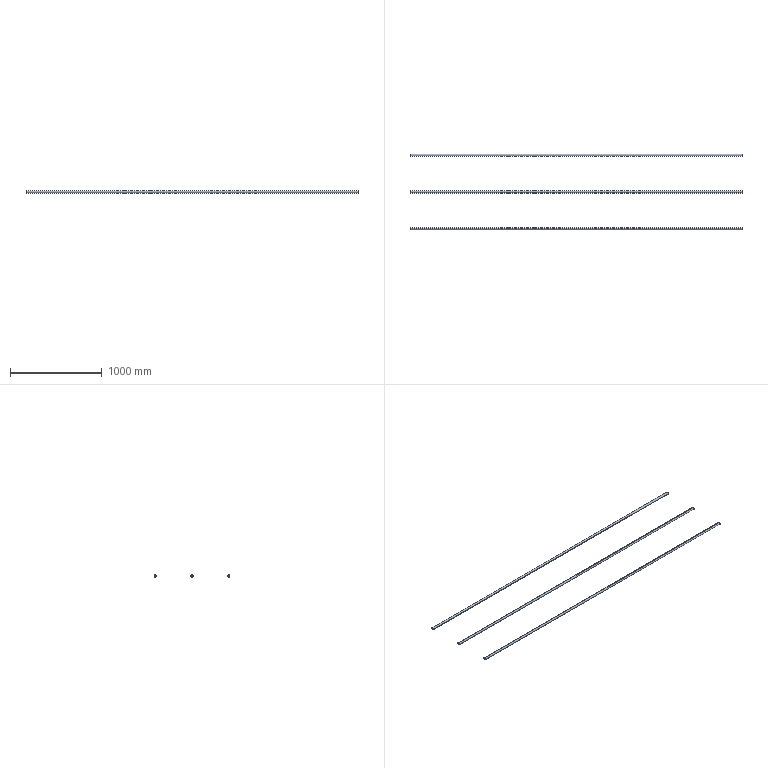Part | STEP file | 粉仓护栏栏杆3_Default<As Machined> | 3 solids | 18 faces | box 3614 x 825 x 25 mm | volume 1200655 mm3 | cylinder 12 | plane 6 | commonest cylinder face diameters 22 x6 25 x6
STEP:
#1=CARTESIAN_POINT('',(0.,0.,0.));
#2=DIRECTION('',(0.,0.,1.));
#3=DIRECTION('',(1.,0.,0.));
#4=AXIS2_PLACEMENT_3D('',#1,#2,#3);
#5=CARTESIAN_POINT('',(-3614.,0.,12.5));
#6=VERTEX_POINT('',#5);
#7=CARTESIAN_POINT('',(-3614.,0.,-12.5));
#8=VERTEX_POINT('',#7);
#9=CARTESIAN_POINT('',(-3614.,0.,0.));
#10=DIRECTION('',(-1.,0.,0.));
#11=DIRECTION('',(0.,-1.,0.));
#12=AXIS2_PLACEMENT_3D('',#9,#10,#11);
#13=CIRCLE('',#12,12.5);
#14=CARTESIAN_POINT('',(-3614.,0.,0.));
#15=DIRECTION('',(1.,0.,0.));
#16=DIRECTION('',(0.,0.,-1.));
#17=AXIS2_PLACEMENT_3D('',#14,#15,#16);
#18=CYLINDRICAL_SURFACE('',#17,12.5);
#19=CARTESIAN_POINT('',(4.712,0.));
#20=DIRECTION('',(-1.,0.));
#21=VECTOR('',#20,1.);
#22=LINE('',#19,#21);
#23=(GEOMETRIC_REPRESENTATION_CONTEXT(2)PARAMETRIC_REPRESENTATION_CONTEXT()REPRESENTATION_CONTEXT('',''));
#24=DEFINITIONAL_REPRESENTATION('',(#22),#23);
#25=PCURVE('',#18,#24);
#26=CARTESIAN_POINT('',(-3614.,0.,0.));
#27=DIRECTION('',(-1.,0.,0.));
#28=DIRECTION('',(0.,-1.,0.));
#29=AXIS2_PLACEMENT_3D('',#26,#27,#28);
#30=PLANE('',#29);
#31=CARTESIAN_POINT('',(0.,0.));
#32=DIRECTION('',(1.,0.));
#33=AXIS2_PLACEMENT_2D('',#31,#32);
#34=CIRCLE('',#33,12.5);
#35=(GEOMETRIC_REPRESENTATION_CONTEXT(2)PARAMETRIC_REPRESENTATION_CONTEXT()REPRESENTATION_CONTEXT('',''));
#36=DEFINITIONAL_REPRESENTATION('',(#34),#35);
#37=PCURVE('',#30,#36);
#38=SURFACE_CURVE('',#13,(#25,#37),.PCURVE_S1.);
#39=EDGE_CURVE('',#6,#8,#38,.T.);
#40=ORIENTED_EDGE('',*,*,#39,.F.);
#41=CARTESIAN_POINT('',(0.,0.,12.5));
#42=VERTEX_POINT('',#41);
#43=CARTESIAN_POINT('',(-3614.,0.,12.5));
#44=DIRECTION('',(1.,0.,0.));
#45=VECTOR('',#44,1.);
#46=LINE('',#43,#45);
#47=CARTESIAN_POINT('',(3.142,0.));
#48=DIRECTION('',(0.,1.));
#49=VECTOR('',#48,1.);
#50=LINE('',#47,#49);
#51=(GEOMETRIC_REPRESENTATION_CONTEXT(2)PARAMETRIC_REPRESENTATION_CONTEXT()REPRESENTATION_CONTEXT('',''));
#52=DEFINITIONAL_REPRESENTATION('',(#50),#51);
#53=PCURVE('',#18,#52);
#54=CARTESIAN_POINT('',(-3614.,0.,0.));
#55=DIRECTION('',(1.,0.,0.));
#56=DIRECTION('',(0.,0.,-1.));
#57=AXIS2_PLACEMENT_3D('',#54,#55,#56);
#58=CYLINDRICAL_SURFACE('',#57,12.5);
#59=CARTESIAN_POINT('',(3.142,0.));
#60=DIRECTION('',(0.,1.));
#61=VECTOR('',#60,1.);
#62=LINE('',#59,#61);
#63=(GEOMETRIC_REPRESENTATION_CONTEXT(2)PARAMETRIC_REPRESENTATION_CONTEXT()REPRESENTATION_CONTEXT('',''));
#64=DEFINITIONAL_REPRESENTATION('',(#62),#63);
#65=PCURVE('',#58,#64);
#66=SURFACE_CURVE('',#46,(#53,#65),.PCURVE_S1.);
#67=EDGE_CURVE('',#6,#42,#66,.T.);
#68=ORIENTED_EDGE('',*,*,#67,.T.);
#69=CARTESIAN_POINT('',(0.,0.,-12.5));
#70=VERTEX_POINT('',#69);
#71=CARTESIAN_POINT('',(0.,0.,0.));
#72=DIRECTION('',(-1.,0.,0.));
#73=DIRECTION('',(0.,-1.,0.));
#74=AXIS2_PLACEMENT_3D('',#71,#72,#73);
#75=CIRCLE('',#74,12.5);
#76=CARTESIAN_POINT('',(4.712,3614.));
#77=DIRECTION('',(-1.,0.));
#78=VECTOR('',#77,1.);
#79=LINE('',#76,#78);
#80=(GEOMETRIC_REPRESENTATION_CONTEXT(2)PARAMETRIC_REPRESENTATION_CONTEXT()REPRESENTATION_CONTEXT('',''));
#81=DEFINITIONAL_REPRESENTATION('',(#79),#80);
#82=PCURVE('',#18,#81);
#83=CARTESIAN_POINT('',(0.,0.,0.));
#84=DIRECTION('',(-1.,0.,0.));
#85=DIRECTION('',(0.,-1.,0.));
#86=AXIS2_PLACEMENT_3D('',#83,#84,#85);
#87=PLANE('',#86);
#88=CARTESIAN_POINT('',(0.,0.));
#89=DIRECTION('',(1.,0.));
#90=AXIS2_PLACEMENT_2D('',#88,#89);
#91=CIRCLE('',#90,12.5);
#92=(GEOMETRIC_REPRESENTATION_CONTEXT(2)PARAMETRIC_REPRESENTATION_CONTEXT()REPRESENTATION_CONTEXT('',''));
#93=DEFINITIONAL_REPRESENTATION('',(#91),#92);
#94=PCURVE('',#87,#93);
#95=SURFACE_CURVE('',#75,(#82,#94),.PCURVE_S1.);
#96=EDGE_CURVE('',#42,#70,#95,.T.);
#97=ORIENTED_EDGE('',*,*,#96,.T.);
#98=CARTESIAN_POINT('',(-3614.,0.,-12.5));
#99=DIRECTION('',(1.,0.,0.));
#100=VECTOR('',#99,1.);
#101=LINE('',#98,#100);
#102=CARTESIAN_POINT('',(0.,0.));
#103=DIRECTION('',(0.,1.));
#104=VECTOR('',#103,1.);
#105=LINE('',#102,#104);
#106=(GEOMETRIC_REPRESENTATION_CONTEXT(2)PARAMETRIC_REPRESENTATION_CONTEXT()REPRESENTATION_CONTEXT('',''));
#107=DEFINITIONAL_REPRESENTATION('',(#105),#106);
#108=PCURVE('',#18,#107);
#109=CARTESIAN_POINT('',(6.283,0.));
#110=DIRECTION('',(0.,1.));
#111=VECTOR('',#110,1.);
#112=LINE('',#109,#111);
#113=(GEOMETRIC_REPRESENTATION_CONTEXT(2)PARAMETRIC_REPRESENTATION_CONTEXT()REPRESENTATION_CONTEXT('',''));
#114=DEFINITIONAL_REPRESENTATION('',(#112),#113);
#115=PCURVE('',#58,#114);
#116=SURFACE_CURVE('',#101,(#108,#115),.PCURVE_S1.);
#117=EDGE_CURVE('',#8,#70,#116,.T.);
#118=ORIENTED_EDGE('',*,*,#117,.F.);
#119=EDGE_LOOP('',(#40,#68,#97,#118));
#120=FACE_BOUND('',#119,.T.);
#121=ADVANCED_FACE('',(#120),#18,.T.);
#122=CARTESIAN_POINT('',(-3614.,0.,-11.));
#123=VERTEX_POINT('',#122);
#124=CARTESIAN_POINT('',(0.,0.,-11.));
#125=VERTEX_POINT('',#124);
#126=CARTESIAN_POINT('',(-3614.,0.,-11.));
#127=DIRECTION('',(1.,0.,0.));
#128=VECTOR('',#127,1.);
#129=LINE('',#126,#128);
#130=CARTESIAN_POINT('',(-3614.,0.,0.));
#131=DIRECTION('',(1.,0.,0.));
#132=DIRECTION('',(0.,0.,-1.));
#133=AXIS2_PLACEMENT_3D('',#130,#131,#132);
#134=CYLINDRICAL_SURFACE('',#133,11.);
#135=CARTESIAN_POINT('',(6.283,0.));
#136=DIRECTION('',(0.,1.));
#137=VECTOR('',#136,1.);
#138=LINE('',#135,#137);
#139=(GEOMETRIC_REPRESENTATION_CONTEXT(2)PARAMETRIC_REPRESENTATION_CONTEXT()REPRESENTATION_CONTEXT('',''));
#140=DEFINITIONAL_REPRESENTATION('',(#138),#139);
#141=PCURVE('',#134,#140);
#142=CARTESIAN_POINT('',(-3614.,0.,0.));
#143=DIRECTION('',(1.,0.,0.));
#144=DIRECTION('',(0.,0.,-1.));
#145=AXIS2_PLACEMENT_3D('',#142,#143,#144);
#146=CYLINDRICAL_SURFACE('',#145,11.);
#147=CARTESIAN_POINT('',(0.,0.));
#148=DIRECTION('',(0.,1.));
#149=VECTOR('',#148,1.);
#150=LINE('',#147,#149);
#151=(GEOMETRIC_REPRESENTATION_CONTEXT(2)PARAMETRIC_REPRESENTATION_CONTEXT()REPRESENTATION_CONTEXT('',''));
#152=DEFINITIONAL_REPRESENTATION('',(#150),#151);
#153=PCURVE('',#146,#152);
#154=SURFACE_CURVE('',#129,(#141,#153),.PCURVE_S1.);
#155=EDGE_CURVE('',#123,#125,#154,.T.);
#156=ORIENTED_EDGE('',*,*,#155,.T.);
#157=CARTESIAN_POINT('',(0.,0.,11.));
#158=VERTEX_POINT('',#157);
#159=CARTESIAN_POINT('',(0.,0.,0.));
#160=DIRECTION('',(-1.,0.,0.));
#161=DIRECTION('',(0.,-1.,0.));
#162=AXIS2_PLACEMENT_3D('',#159,#160,#161);
#163=CIRCLE('',#162,11.);
#164=CARTESIAN_POINT('',(10.996,3614.));
#165=DIRECTION('',(-1.,0.));
#166=VECTOR('',#165,1.);
#167=LINE('',#164,#166);
#168=(GEOMETRIC_REPRESENTATION_CONTEXT(2)PARAMETRIC_REPRESENTATION_CONTEXT()REPRESENTATION_CONTEXT('',''));
#169=DEFINITIONAL_REPRESENTATION('',(#167),#168);
#170=PCURVE('',#134,#169);
#171=CARTESIAN_POINT('',(0.,0.));
#172=DIRECTION('',(1.,0.));
#173=AXIS2_PLACEMENT_2D('',#171,#172);
#174=CIRCLE('',#173,11.);
#175=(GEOMETRIC_REPRESENTATION_CONTEXT(2)PARAMETRIC_REPRESENTATION_CONTEXT()REPRESENTATION_CONTEXT('',''));
#176=DEFINITIONAL_REPRESENTATION('',(#174),#175);
#177=PCURVE('',#87,#176);
#178=SURFACE_CURVE('',#163,(#170,#177),.PCURVE_S1.);
#179=EDGE_CURVE('',#125,#158,#178,.T.);
#180=ORIENTED_EDGE('',*,*,#179,.T.);
#181=CARTESIAN_POINT('',(-3614.,0.,11.));
#182=VERTEX_POINT('',#181);
#183=CARTESIAN_POINT('',(-3614.,0.,11.));
#184=DIRECTION('',(1.,0.,0.));
#185=VECTOR('',#184,1.);
#186=LINE('',#183,#185);
#187=CARTESIAN_POINT('',(3.142,0.));
#188=DIRECTION('',(0.,1.));
#189=VECTOR('',#188,1.);
#190=LINE('',#187,#189);
#191=(GEOMETRIC_REPRESENTATION_CONTEXT(2)PARAMETRIC_REPRESENTATION_CONTEXT()REPRESENTATION_CONTEXT('',''));
#192=DEFINITIONAL_REPRESENTATION('',(#190),#191);
#193=PCURVE('',#134,#192);
#194=CARTESIAN_POINT('',(3.142,0.));
#195=DIRECTION('',(0.,1.));
#196=VECTOR('',#195,1.);
#197=LINE('',#194,#196);
#198=(GEOMETRIC_REPRESENTATION_CONTEXT(2)PARAMETRIC_REPRESENTATION_CONTEXT()REPRESENTATION_CONTEXT('',''));
#199=DEFINITIONAL_REPRESENTATION('',(#197),#198);
#200=PCURVE('',#146,#199);
#201=SURFACE_CURVE('',#186,(#193,#200),.PCURVE_S1.);
#202=EDGE_CURVE('',#182,#158,#201,.T.);
#203=ORIENTED_EDGE('',*,*,#202,.F.);
#204=CARTESIAN_POINT('',(-3614.,0.,0.));
#205=DIRECTION('',(-1.,0.,0.));
#206=DIRECTION('',(0.,-1.,0.));
#207=AXIS2_PLACEMENT_3D('',#204,#205,#206);
#208=CIRCLE('',#207,11.);
#209=CARTESIAN_POINT('',(10.996,0.));
#210=DIRECTION('',(-1.,0.));
#211=VECTOR('',#210,1.);
#212=LINE('',#209,#211);
#213=(GEOMETRIC_REPRESENTATION_CONTEXT(2)PARAMETRIC_REPRESENTATION_CONTEXT()REPRESENTATION_CONTEXT('',''));
#214=DEFINITIONAL_REPRESENTATION('',(#212),#213);
#215=PCURVE('',#134,#214);
#216=CARTESIAN_POINT('',(0.,0.));
#217=DIRECTION('',(1.,0.));
#218=AXIS2_PLACEMENT_2D('',#216,#217);
#219=CIRCLE('',#218,11.);
#220=(GEOMETRIC_REPRESENTATION_CONTEXT(2)PARAMETRIC_REPRESENTATION_CONTEXT()REPRESENTATION_CONTEXT('',''));
#221=DEFINITIONAL_REPRESENTATION('',(#219),#220);
#222=PCURVE('',#30,#221);
#223=SURFACE_CURVE('',#208,(#215,#222),.PCURVE_S1.);
#224=EDGE_CURVE('',#123,#182,#223,.T.);
#225=ORIENTED_EDGE('',*,*,#224,.F.);
#226=EDGE_LOOP('',(#156,#180,#203,#225));
#227=FACE_BOUND('',#226,.F.);
#228=ADVANCED_FACE('',(#227),#134,.F.);
#229=CARTESIAN_POINT('',(0.,0.,0.));
#230=DIRECTION('',(-1.,0.,0.));
#231=DIRECTION('',(0.,-1.,0.));
#232=AXIS2_PLACEMENT_3D('',#229,#230,#231);
#233=CIRCLE('',#232,11.);
#234=CARTESIAN_POINT('',(4.712,3614.));
#235=DIRECTION('',(-1.,0.));
#236=VECTOR('',#235,1.);
#237=LINE('',#234,#236);
#238=(GEOMETRIC_REPRESENTATION_CONTEXT(2)PARAMETRIC_REPRESENTATION_CONTEXT()REPRESENTATION_CONTEXT('',''));
#239=DEFINITIONAL_REPRESENTATION('',(#237),#238);
#240=PCURVE('',#146,#239);
#241=CARTESIAN_POINT('',(0.,0.));
#242=DIRECTION('',(1.,0.));
#243=AXIS2_PLACEMENT_2D('',#241,#242);
#244=CIRCLE('',#243,11.);
#245=(GEOMETRIC_REPRESENTATION_CONTEXT(2)PARAMETRIC_REPRESENTATION_CONTEXT()REPRESENTATION_CONTEXT('',''));
#246=DEFINITIONAL_REPRESENTATION('',(#244),#245);
#247=PCURVE('',#87,#246);
#248=SURFACE_CURVE('',#233,(#240,#247),.PCURVE_S1.);
#249=EDGE_CURVE('',#158,#125,#248,.T.);
#250=ORIENTED_EDGE('',*,*,#249,.T.);
#251=ORIENTED_EDGE('',*,*,#155,.F.);
#252=CARTESIAN_POINT('',(-3614.,0.,0.));
#253=DIRECTION('',(-1.,0.,0.));
#254=DIRECTION('',(0.,-1.,0.));
#255=AXIS2_PLACEMENT_3D('',#252,#253,#254);
#256=CIRCLE('',#255,11.);
#257=CARTESIAN_POINT('',(4.712,0.));
#258=DIRECTION('',(-1.,0.));
#259=VECTOR('',#258,1.);
#260=LINE('',#257,#259);
#261=(GEOMETRIC_REPRESENTATION_CONTEXT(2)PARAMETRIC_REPRESENTATION_CONTEXT()REPRESENTATION_CONTEXT('',''));
#262=DEFINITIONAL_REPRESENTATION('',(#260),#261);
#263=PCURVE('',#146,#262);
#264=CARTESIAN_POINT('',(0.,0.));
#265=DIRECTION('',(1.,0.));
#266=AXIS2_PLACEMENT_2D('',#264,#265);
#267=CIRCLE('',#266,11.);
#268=(GEOMETRIC_REPRESENTATION_CONTEXT(2)PARAMETRIC_REPRESENTATION_CONTEXT()REPRESENTATION_CONTEXT('',''));
#269=DEFINITIONAL_REPRESENTATION('',(#267),#268);
#270=PCURVE('',#30,#269);
#271=SURFACE_CURVE('',#256,(#263,#270),.PCURVE_S1.);
#272=EDGE_CURVE('',#182,#123,#271,.T.);
#273=ORIENTED_EDGE('',*,*,#272,.F.);
#274=ORIENTED_EDGE('',*,*,#202,.T.);
#275=EDGE_LOOP('',(#250,#251,#273,#274));
#276=FACE_BOUND('',#275,.F.);
#277=ADVANCED_FACE('',(#276),#146,.F.);
#278=ORIENTED_EDGE('',*,*,#67,.F.);
#279=CARTESIAN_POINT('',(-3614.,0.,0.));
#280=DIRECTION('',(-1.,0.,0.));
#281=DIRECTION('',(0.,-1.,0.));
#282=AXIS2_PLACEMENT_3D('',#279,#280,#281);
#283=CIRCLE('',#282,12.5);
#284=CARTESIAN_POINT('',(10.996,0.));
#285=DIRECTION('',(-1.,0.));
#286=VECTOR('',#285,1.);
#287=LINE('',#284,#286);
#288=(GEOMETRIC_REPRESENTATION_CONTEXT(2)PARAMETRIC_REPRESENTATION_CONTEXT()REPRESENTATION_CONTEXT('',''));
#289=DEFINITIONAL_REPRESENTATION('',(#287),#288);
#290=PCURVE('',#58,#289);
#291=CARTESIAN_POINT('',(0.,0.));
#292=DIRECTION('',(1.,0.));
#293=AXIS2_PLACEMENT_2D('',#291,#292);
#294=CIRCLE('',#293,12.5);
#295=(GEOMETRIC_REPRESENTATION_CONTEXT(2)PARAMETRIC_REPRESENTATION_CONTEXT()REPRESENTATION_CONTEXT('',''));
#296=DEFINITIONAL_REPRESENTATION('',(#294),#295);
#297=PCURVE('',#30,#296);
#298=SURFACE_CURVE('',#283,(#290,#297),.PCURVE_S1.);
#299=EDGE_CURVE('',#8,#6,#298,.T.);
#300=ORIENTED_EDGE('',*,*,#299,.F.);
#301=ORIENTED_EDGE('',*,*,#117,.T.);
#302=CARTESIAN_POINT('',(0.,0.,0.));
#303=DIRECTION('',(-1.,0.,0.));
#304=DIRECTION('',(0.,-1.,0.));
#305=AXIS2_PLACEMENT_3D('',#302,#303,#304);
#306=CIRCLE('',#305,12.5);
#307=CARTESIAN_POINT('',(10.996,3614.));
#308=DIRECTION('',(-1.,0.));
#309=VECTOR('',#308,1.);
#310=LINE('',#307,#309);
#311=(GEOMETRIC_REPRESENTATION_CONTEXT(2)PARAMETRIC_REPRESENTATION_CONTEXT()REPRESENTATION_CONTEXT('',''));
#312=DEFINITIONAL_REPRESENTATION('',(#310),#311);
#313=PCURVE('',#58,#312);
#314=CARTESIAN_POINT('',(0.,0.));
#315=DIRECTION('',(1.,0.));
#316=AXIS2_PLACEMENT_2D('',#314,#315);
#317=CIRCLE('',#316,12.5);
#318=(GEOMETRIC_REPRESENTATION_CONTEXT(2)PARAMETRIC_REPRESENTATION_CONTEXT()REPRESENTATION_CONTEXT('',''));
#319=DEFINITIONAL_REPRESENTATION('',(#317),#318);
#320=PCURVE('',#87,#319);
#321=SURFACE_CURVE('',#306,(#313,#320),.PCURVE_S1.);
#322=EDGE_CURVE('',#70,#42,#321,.T.);
#323=ORIENTED_EDGE('',*,*,#322,.T.);
#324=EDGE_LOOP('',(#278,#300,#301,#323));
#325=FACE_BOUND('',#324,.T.);
#326=ADVANCED_FACE('',(#325),#58,.T.);
#327=ORIENTED_EDGE('',*,*,#224,.F.);
#328=ORIENTED_EDGE('',*,*,#272,.F.);
#329=EDGE_LOOP('',(#327,#328));
#330=FACE_BOUND('',#329,.T.);
#331=ORIENTED_EDGE('',*,*,#299,.T.);
#332=ORIENTED_EDGE('',*,*,#39,.T.);
#333=EDGE_LOOP('',(#331,#332));
#334=FACE_BOUND('',#333,.T.);
#335=ADVANCED_FACE('',(#330,#334),#30,.T.);
#336=ORIENTED_EDGE('',*,*,#179,.T.);
#337=ORIENTED_EDGE('',*,*,#249,.T.);
#338=EDGE_LOOP('',(#336,#337));
#339=FACE_BOUND('',#338,.T.);
#340=ORIENTED_EDGE('',*,*,#322,.F.);
#341=ORIENTED_EDGE('',*,*,#96,.F.);
#342=EDGE_LOOP('',(#340,#341));
#343=FACE_BOUND('',#342,.T.);
#344=ADVANCED_FACE('',(#339,#343),#87,.F.);
#345=CLOSED_SHELL('',(#121,#228,#277,#326,#335,#344));
#346=MANIFOLD_SOLID_BREP('',#345);
#347=CARTESIAN_POINT('',(-3614.,787.5,0.));
#348=VERTEX_POINT('',#347);
#349=CARTESIAN_POINT('',(-3614.,812.5,0.));
#350=VERTEX_POINT('',#349);
#351=CARTESIAN_POINT('',(-3614.,800.,0.));
#352=DIRECTION('',(-1.,0.,0.));
#353=DIRECTION('',(0.,-1.,0.));
#354=AXIS2_PLACEMENT_3D('',#351,#352,#353);
#355=CIRCLE('',#354,12.5);
#356=CARTESIAN_POINT('',(-3614.,800.,0.));
#357=DIRECTION('',(1.,0.,0.));
#358=DIRECTION('',(0.,1.,0.));
#359=AXIS2_PLACEMENT_3D('',#356,#357,#358);
#360=CYLINDRICAL_SURFACE('',#359,12.5);
#361=CARTESIAN_POINT('',(3.142,0.));
#362=DIRECTION('',(-1.,0.));
#363=VECTOR('',#362,1.);
#364=LINE('',#361,#363);
#365=(GEOMETRIC_REPRESENTATION_CONTEXT(2)PARAMETRIC_REPRESENTATION_CONTEXT()REPRESENTATION_CONTEXT('',''));
#366=DEFINITIONAL_REPRESENTATION('',(#364),#365);
#367=PCURVE('',#360,#366);
#368=CARTESIAN_POINT('',(-3614.,800.,0.));
#369=DIRECTION('',(-1.,0.,0.));
#370=DIRECTION('',(0.,-1.,0.));
#371=AXIS2_PLACEMENT_3D('',#368,#369,#370);
#372=PLANE('',#371);
#373=CARTESIAN_POINT('',(0.,0.));
#374=DIRECTION('',(1.,0.));
#375=AXIS2_PLACEMENT_2D('',#373,#374);
#376=CIRCLE('',#375,12.5);
#377=(GEOMETRIC_REPRESENTATION_CONTEXT(2)PARAMETRIC_REPRESENTATION_CONTEXT()REPRESENTATION_CONTEXT('',''));
#378=DEFINITIONAL_REPRESENTATION('',(#376),#377);
#379=PCURVE('',#372,#378);
#380=SURFACE_CURVE('',#355,(#367,#379),.PCURVE_S1.);
#381=EDGE_CURVE('',#348,#350,#380,.T.);
#382=ORIENTED_EDGE('',*,*,#381,.F.);
#383=CARTESIAN_POINT('',(0.,787.5,0.));
#384=VERTEX_POINT('',#383);
#385=CARTESIAN_POINT('',(-3614.,787.5,0.));
#386=DIRECTION('',(1.,0.,0.));
#387=VECTOR('',#386,1.);
#388=LINE('',#385,#387);
#389=CARTESIAN_POINT('',(3.142,0.));
#390=DIRECTION('',(0.,1.));
#391=VECTOR('',#390,1.);
#392=LINE('',#389,#391);
#393=(GEOMETRIC_REPRESENTATION_CONTEXT(2)PARAMETRIC_REPRESENTATION_CONTEXT()REPRESENTATION_CONTEXT('',''));
#394=DEFINITIONAL_REPRESENTATION('',(#392),#393);
#395=PCURVE('',#360,#394);
#396=CARTESIAN_POINT('',(-3614.,800.,0.));
#397=DIRECTION('',(1.,0.,0.));
#398=DIRECTION('',(0.,1.,0.));
#399=AXIS2_PLACEMENT_3D('',#396,#397,#398);
#400=CYLINDRICAL_SURFACE('',#399,12.5);
#401=CARTESIAN_POINT('',(3.142,0.));
#402=DIRECTION('',(0.,1.));
#403=VECTOR('',#402,1.);
#404=LINE('',#401,#403);
#405=(GEOMETRIC_REPRESENTATION_CONTEXT(2)PARAMETRIC_REPRESENTATION_CONTEXT()REPRESENTATION_CONTEXT('',''));
#406=DEFINITIONAL_REPRESENTATION('',(#404),#405);
#407=PCURVE('',#400,#406);
#408=SURFACE_CURVE('',#388,(#395,#407),.PCURVE_S1.);
#409=EDGE_CURVE('',#348,#384,#408,.T.);
#410=ORIENTED_EDGE('',*,*,#409,.T.);
#411=CARTESIAN_POINT('',(0.,812.5,0.));
#412=VERTEX_POINT('',#411);
#413=CARTESIAN_POINT('',(0.,800.,0.));
#414=DIRECTION('',(-1.,0.,0.));
#415=DIRECTION('',(0.,-1.,0.));
#416=AXIS2_PLACEMENT_3D('',#413,#414,#415);
#417=CIRCLE('',#416,12.5);
#418=CARTESIAN_POINT('',(3.142,3614.));
#419=DIRECTION('',(-1.,0.));
#420=VECTOR('',#419,1.);
#421=LINE('',#418,#420);
#422=(GEOMETRIC_REPRESENTATION_CONTEXT(2)PARAMETRIC_REPRESENTATION_CONTEXT()REPRESENTATION_CONTEXT('',''));
#423=DEFINITIONAL_REPRESENTATION('',(#421),#422);
#424=PCURVE('',#360,#423);
#425=CARTESIAN_POINT('',(0.,800.,0.));
#426=DIRECTION('',(-1.,0.,0.));
#427=DIRECTION('',(0.,-1.,0.));
#428=AXIS2_PLACEMENT_3D('',#425,#426,#427);
#429=PLANE('',#428);
#430=CARTESIAN_POINT('',(0.,0.));
#431=DIRECTION('',(1.,0.));
#432=AXIS2_PLACEMENT_2D('',#430,#431);
#433=CIRCLE('',#432,12.5);
#434=(GEOMETRIC_REPRESENTATION_CONTEXT(2)PARAMETRIC_REPRESENTATION_CONTEXT()REPRESENTATION_CONTEXT('',''));
#435=DEFINITIONAL_REPRESENTATION('',(#433),#434);
#436=PCURVE('',#429,#435);
#437=SURFACE_CURVE('',#417,(#424,#436),.PCURVE_S1.);
#438=EDGE_CURVE('',#384,#412,#437,.T.);
#439=ORIENTED_EDGE('',*,*,#438,.T.);
#440=CARTESIAN_POINT('',(-3614.,812.5,0.));
#441=DIRECTION('',(1.,0.,0.));
#442=VECTOR('',#441,1.);
#443=LINE('',#440,#442);
#444=CARTESIAN_POINT('',(0.,0.));
#445=DIRECTION('',(0.,1.));
#446=VECTOR('',#445,1.);
#447=LINE('',#444,#446);
#448=(GEOMETRIC_REPRESENTATION_CONTEXT(2)PARAMETRIC_REPRESENTATION_CONTEXT()REPRESENTATION_CONTEXT('',''));
#449=DEFINITIONAL_REPRESENTATION('',(#447),#448);
#450=PCURVE('',#360,#449);
#451=CARTESIAN_POINT('',(6.283,0.));
#452=DIRECTION('',(0.,1.));
#453=VECTOR('',#452,1.);
#454=LINE('',#451,#453);
#455=(GEOMETRIC_REPRESENTATION_CONTEXT(2)PARAMETRIC_REPRESENTATION_CONTEXT()REPRESENTATION_CONTEXT('',''));
#456=DEFINITIONAL_REPRESENTATION('',(#454),#455);
#457=PCURVE('',#400,#456);
#458=SURFACE_CURVE('',#443,(#450,#457),.PCURVE_S1.);
#459=EDGE_CURVE('',#350,#412,#458,.T.);
#460=ORIENTED_EDGE('',*,*,#459,.F.);
#461=EDGE_LOOP('',(#382,#410,#439,#460));
#462=FACE_BOUND('',#461,.T.);
#463=ADVANCED_FACE('',(#462),#360,.T.);
#464=CARTESIAN_POINT('',(-3614.,811.,0.));
#465=VERTEX_POINT('',#464);
#466=CARTESIAN_POINT('',(0.,811.,0.));
#467=VERTEX_POINT('',#466);
#468=CARTESIAN_POINT('',(-3614.,811.,0.));
#469=DIRECTION('',(1.,0.,0.));
#470=VECTOR('',#469,1.);
#471=LINE('',#468,#470);
#472=CARTESIAN_POINT('',(-3614.,800.,0.));
#473=DIRECTION('',(1.,0.,0.));
#474=DIRECTION('',(0.,1.,0.));
#475=AXIS2_PLACEMENT_3D('',#472,#473,#474);
#476=CYLINDRICAL_SURFACE('',#475,11.);
#477=CARTESIAN_POINT('',(6.283,0.));
#478=DIRECTION('',(0.,1.));
#479=VECTOR('',#478,1.);
#480=LINE('',#477,#479);
#481=(GEOMETRIC_REPRESENTATION_CONTEXT(2)PARAMETRIC_REPRESENTATION_CONTEXT()REPRESENTATION_CONTEXT('',''));
#482=DEFINITIONAL_REPRESENTATION('',(#480),#481);
#483=PCURVE('',#476,#482);
#484=CARTESIAN_POINT('',(-3614.,800.,0.));
#485=DIRECTION('',(1.,0.,0.));
#486=DIRECTION('',(0.,1.,0.));
#487=AXIS2_PLACEMENT_3D('',#484,#485,#486);
#488=CYLINDRICAL_SURFACE('',#487,11.);
#489=CARTESIAN_POINT('',(0.,0.));
#490=DIRECTION('',(0.,1.));
#491=VECTOR('',#490,1.);
#492=LINE('',#489,#491);
#493=(GEOMETRIC_REPRESENTATION_CONTEXT(2)PARAMETRIC_REPRESENTATION_CONTEXT()REPRESENTATION_CONTEXT('',''));
#494=DEFINITIONAL_REPRESENTATION('',(#492),#493);
#495=PCURVE('',#488,#494);
#496=SURFACE_CURVE('',#471,(#483,#495),.PCURVE_S1.);
#497=EDGE_CURVE('',#465,#467,#496,.T.);
#498=ORIENTED_EDGE('',*,*,#497,.T.);
#499=CARTESIAN_POINT('',(0.,789.,0.));
#500=VERTEX_POINT('',#499);
#501=CARTESIAN_POINT('',(0.,800.,0.));
#502=DIRECTION('',(-1.,0.,0.));
#503=DIRECTION('',(0.,-1.,0.));
#504=AXIS2_PLACEMENT_3D('',#501,#502,#503);
#505=CIRCLE('',#504,11.);
#506=CARTESIAN_POINT('',(9.425,3614.));
#507=DIRECTION('',(-1.,0.));
#508=VECTOR('',#507,1.);
#509=LINE('',#506,#508);
#510=(GEOMETRIC_REPRESENTATION_CONTEXT(2)PARAMETRIC_REPRESENTATION_CONTEXT()REPRESENTATION_CONTEXT('',''));
#511=DEFINITIONAL_REPRESENTATION('',(#509),#510);
#512=PCURVE('',#476,#511);
#513=CARTESIAN_POINT('',(0.,0.));
#514=DIRECTION('',(1.,0.));
#515=AXIS2_PLACEMENT_2D('',#513,#514);
#516=CIRCLE('',#515,11.);
#517=(GEOMETRIC_REPRESENTATION_CONTEXT(2)PARAMETRIC_REPRESENTATION_CONTEXT()REPRESENTATION_CONTEXT('',''));
#518=DEFINITIONAL_REPRESENTATION('',(#516),#517);
#519=PCURVE('',#429,#518);
#520=SURFACE_CURVE('',#505,(#512,#519),.PCURVE_S1.);
#521=EDGE_CURVE('',#467,#500,#520,.T.);
#522=ORIENTED_EDGE('',*,*,#521,.T.);
#523=CARTESIAN_POINT('',(-3614.,789.,0.));
#524=VERTEX_POINT('',#523);
#525=CARTESIAN_POINT('',(-3614.,789.,0.));
#526=DIRECTION('',(1.,0.,0.));
#527=VECTOR('',#526,1.);
#528=LINE('',#525,#527);
#529=CARTESIAN_POINT('',(3.142,0.));
#530=DIRECTION('',(0.,1.));
#531=VECTOR('',#530,1.);
#532=LINE('',#529,#531);
#533=(GEOMETRIC_REPRESENTATION_CONTEXT(2)PARAMETRIC_REPRESENTATION_CONTEXT()REPRESENTATION_CONTEXT('',''));
#534=DEFINITIONAL_REPRESENTATION('',(#532),#533);
#535=PCURVE('',#476,#534);
#536=CARTESIAN_POINT('',(3.142,0.));
#537=DIRECTION('',(0.,1.));
#538=VECTOR('',#537,1.);
#539=LINE('',#536,#538);
#540=(GEOMETRIC_REPRESENTATION_CONTEXT(2)PARAMETRIC_REPRESENTATION_CONTEXT()REPRESENTATION_CONTEXT('',''));
#541=DEFINITIONAL_REPRESENTATION('',(#539),#540);
#542=PCURVE('',#488,#541);
#543=SURFACE_CURVE('',#528,(#535,#542),.PCURVE_S1.);
#544=EDGE_CURVE('',#524,#500,#543,.T.);
#545=ORIENTED_EDGE('',*,*,#544,.F.);
#546=CARTESIAN_POINT('',(-3614.,800.,0.));
#547=DIRECTION('',(-1.,0.,0.));
#548=DIRECTION('',(0.,-1.,0.));
#549=AXIS2_PLACEMENT_3D('',#546,#547,#548);
#550=CIRCLE('',#549,11.);
#551=CARTESIAN_POINT('',(9.425,0.));
#552=DIRECTION('',(-1.,0.));
#553=VECTOR('',#552,1.);
#554=LINE('',#551,#553);
#555=(GEOMETRIC_REPRESENTATION_CONTEXT(2)PARAMETRIC_REPRESENTATION_CONTEXT()REPRESENTATION_CONTEXT('',''));
#556=DEFINITIONAL_REPRESENTATION('',(#554),#555);
#557=PCURVE('',#476,#556);
#558=CARTESIAN_POINT('',(0.,0.));
#559=DIRECTION('',(1.,0.));
#560=AXIS2_PLACEMENT_2D('',#558,#559);
#561=CIRCLE('',#560,11.);
#562=(GEOMETRIC_REPRESENTATION_CONTEXT(2)PARAMETRIC_REPRESENTATION_CONTEXT()REPRESENTATION_CONTEXT('',''));
#563=DEFINITIONAL_REPRESENTATION('',(#561),#562);
#564=PCURVE('',#372,#563);
#565=SURFACE_CURVE('',#550,(#557,#564),.PCURVE_S1.);
#566=EDGE_CURVE('',#465,#524,#565,.T.);
#567=ORIENTED_EDGE('',*,*,#566,.F.);
#568=EDGE_LOOP('',(#498,#522,#545,#567));
#569=FACE_BOUND('',#568,.F.);
#570=ADVANCED_FACE('',(#569),#476,.F.);
#571=CARTESIAN_POINT('',(0.,800.,0.));
#572=DIRECTION('',(-1.,0.,0.));
#573=DIRECTION('',(0.,-1.,0.));
#574=AXIS2_PLACEMENT_3D('',#571,#572,#573);
#575=CIRCLE('',#574,11.);
#576=CARTESIAN_POINT('',(3.142,3614.));
#577=DIRECTION('',(-1.,0.));
#578=VECTOR('',#577,1.);
#579=LINE('',#576,#578);
#580=(GEOMETRIC_REPRESENTATION_CONTEXT(2)PARAMETRIC_REPRESENTATION_CONTEXT()REPRESENTATION_CONTEXT('',''));
#581=DEFINITIONAL_REPRESENTATION('',(#579),#580);
#582=PCURVE('',#488,#581);
#583=CARTESIAN_POINT('',(0.,0.));
#584=DIRECTION('',(1.,0.));
#585=AXIS2_PLACEMENT_2D('',#583,#584);
#586=CIRCLE('',#585,11.);
#587=(GEOMETRIC_REPRESENTATION_CONTEXT(2)PARAMETRIC_REPRESENTATION_CONTEXT()REPRESENTATION_CONTEXT('',''));
#588=DEFINITIONAL_REPRESENTATION('',(#586),#587);
#589=PCURVE('',#429,#588);
#590=SURFACE_CURVE('',#575,(#582,#589),.PCURVE_S1.);
#591=EDGE_CURVE('',#500,#467,#590,.T.);
#592=ORIENTED_EDGE('',*,*,#591,.T.);
#593=ORIENTED_EDGE('',*,*,#497,.F.);
#594=CARTESIAN_POINT('',(-3614.,800.,0.));
#595=DIRECTION('',(-1.,0.,0.));
#596=DIRECTION('',(0.,-1.,0.));
#597=AXIS2_PLACEMENT_3D('',#594,#595,#596);
#598=CIRCLE('',#597,11.);
#599=CARTESIAN_POINT('',(3.142,0.));
#600=DIRECTION('',(-1.,0.));
#601=VECTOR('',#600,1.);
#602=LINE('',#599,#601);
#603=(GEOMETRIC_REPRESENTATION_CONTEXT(2)PARAMETRIC_REPRESENTATION_CONTEXT()REPRESENTATION_CONTEXT('',''));
#604=DEFINITIONAL_REPRESENTATION('',(#602),#603);
#605=PCURVE('',#488,#604);
#606=CARTESIAN_POINT('',(0.,0.));
#607=DIRECTION('',(1.,0.));
#608=AXIS2_PLACEMENT_2D('',#606,#607);
#609=CIRCLE('',#608,11.);
#610=(GEOMETRIC_REPRESENTATION_CONTEXT(2)PARAMETRIC_REPRESENTATION_CONTEXT()REPRESENTATION_CONTEXT('',''));
#611=DEFINITIONAL_REPRESENTATION('',(#609),#610);
#612=PCURVE('',#372,#611);
#613=SURFACE_CURVE('',#598,(#605,#612),.PCURVE_S1.);
#614=EDGE_CURVE('',#524,#465,#613,.T.);
#615=ORIENTED_EDGE('',*,*,#614,.F.);
#616=ORIENTED_EDGE('',*,*,#544,.T.);
#617=EDGE_LOOP('',(#592,#593,#615,#616));
#618=FACE_BOUND('',#617,.F.);
#619=ADVANCED_FACE('',(#618),#488,.F.);
#620=ORIENTED_EDGE('',*,*,#409,.F.);
#621=CARTESIAN_POINT('',(-3614.,800.,0.));
#622=DIRECTION('',(-1.,0.,0.));
#623=DIRECTION('',(0.,-1.,0.));
#624=AXIS2_PLACEMENT_3D('',#621,#622,#623);
#625=CIRCLE('',#624,12.5);
#626=CARTESIAN_POINT('',(9.425,0.));
#627=DIRECTION('',(-1.,0.));
#628=VECTOR('',#627,1.);
#629=LINE('',#626,#628);
#630=(GEOMETRIC_REPRESENTATION_CONTEXT(2)PARAMETRIC_REPRESENTATION_CONTEXT()REPRESENTATION_CONTEXT('',''));
#631=DEFINITIONAL_REPRESENTATION('',(#629),#630);
#632=PCURVE('',#400,#631);
#633=CARTESIAN_POINT('',(0.,0.));
#634=DIRECTION('',(1.,0.));
#635=AXIS2_PLACEMENT_2D('',#633,#634);
#636=CIRCLE('',#635,12.5);
#637=(GEOMETRIC_REPRESENTATION_CONTEXT(2)PARAMETRIC_REPRESENTATION_CONTEXT()REPRESENTATION_CONTEXT('',''));
#638=DEFINITIONAL_REPRESENTATION('',(#636),#637);
#639=PCURVE('',#372,#638);
#640=SURFACE_CURVE('',#625,(#632,#639),.PCURVE_S1.);
#641=EDGE_CURVE('',#350,#348,#640,.T.);
#642=ORIENTED_EDGE('',*,*,#641,.F.);
#643=ORIENTED_EDGE('',*,*,#459,.T.);
#644=CARTESIAN_POINT('',(0.,800.,0.));
#645=DIRECTION('',(-1.,0.,0.));
#646=DIRECTION('',(0.,-1.,0.));
#647=AXIS2_PLACEMENT_3D('',#644,#645,#646);
#648=CIRCLE('',#647,12.5);
#649=CARTESIAN_POINT('',(9.425,3614.));
#650=DIRECTION('',(-1.,0.));
#651=VECTOR('',#650,1.);
#652=LINE('',#649,#651);
#653=(GEOMETRIC_REPRESENTATION_CONTEXT(2)PARAMETRIC_REPRESENTATION_CONTEXT()REPRESENTATION_CONTEXT('',''));
#654=DEFINITIONAL_REPRESENTATION('',(#652),#653);
#655=PCURVE('',#400,#654);
#656=CARTESIAN_POINT('',(0.,0.));
#657=DIRECTION('',(1.,0.));
#658=AXIS2_PLACEMENT_2D('',#656,#657);
#659=CIRCLE('',#658,12.5);
#660=(GEOMETRIC_REPRESENTATION_CONTEXT(2)PARAMETRIC_REPRESENTATION_CONTEXT()REPRESENTATION_CONTEXT('',''));
#661=DEFINITIONAL_REPRESENTATION('',(#659),#660);
#662=PCURVE('',#429,#661);
#663=SURFACE_CURVE('',#648,(#655,#662),.PCURVE_S1.);
#664=EDGE_CURVE('',#412,#384,#663,.T.);
#665=ORIENTED_EDGE('',*,*,#664,.T.);
#666=EDGE_LOOP('',(#620,#642,#643,#665));
#667=FACE_BOUND('',#666,.T.);
#668=ADVANCED_FACE('',(#667),#400,.T.);
#669=ORIENTED_EDGE('',*,*,#566,.F.);
#670=ORIENTED_EDGE('',*,*,#614,.F.);
#671=EDGE_LOOP('',(#669,#670));
#672=FACE_BOUND('',#671,.T.);
#673=ORIENTED_EDGE('',*,*,#641,.T.);
#674=ORIENTED_EDGE('',*,*,#381,.T.);
#675=EDGE_LOOP('',(#673,#674));
#676=FACE_BOUND('',#675,.T.);
#677=ADVANCED_FACE('',(#672,#676),#372,.T.);
#678=ORIENTED_EDGE('',*,*,#521,.T.);
#679=ORIENTED_EDGE('',*,*,#591,.T.);
#680=EDGE_LOOP('',(#678,#679));
#681=FACE_BOUND('',#680,.T.);
#682=ORIENTED_EDGE('',*,*,#664,.F.);
#683=ORIENTED_EDGE('',*,*,#438,.F.);
#684=EDGE_LOOP('',(#682,#683));
#685=FACE_BOUND('',#684,.T.);
#686=ADVANCED_FACE('',(#681,#685),#429,.F.);
#687=CLOSED_SHELL('',(#463,#570,#619,#668,#677,#686));
#688=MANIFOLD_SOLID_BREP('',#687);
#689=CARTESIAN_POINT('',(0.,400.,-12.5));
#690=VERTEX_POINT('',#689);
#691=CARTESIAN_POINT('',(0.,400.,12.5));
#692=VERTEX_POINT('',#691);
#693=CARTESIAN_POINT('',(0.,400.,0.));
#694=DIRECTION('',(1.,0.,0.));
#695=DIRECTION('',(0.,1.,0.));
#696=AXIS2_PLACEMENT_3D('',#693,#694,#695);
#697=CIRCLE('',#696,12.5);
#698=CARTESIAN_POINT('',(0.,400.,0.));
#699=DIRECTION('',(-1.,0.,0.));
#700=DIRECTION('',(0.,0.,1.));
#701=AXIS2_PLACEMENT_3D('',#698,#699,#700);
#702=CYLINDRICAL_SURFACE('',#701,12.5);
#703=CARTESIAN_POINT('',(7.854,0.));
#704=DIRECTION('',(-1.,0.));
#705=VECTOR('',#704,1.);
#706=LINE('',#703,#705);
#707=(GEOMETRIC_REPRESENTATION_CONTEXT(2)PARAMETRIC_REPRESENTATION_CONTEXT()REPRESENTATION_CONTEXT('',''));
#708=DEFINITIONAL_REPRESENTATION('',(#706),#707);
#709=PCURVE('',#702,#708);
#710=CARTESIAN_POINT('',(0.,400.,0.));
#711=DIRECTION('',(1.,0.,0.));
#712=DIRECTION('',(0.,1.,0.));
#713=AXIS2_PLACEMENT_3D('',#710,#711,#712);
#714=PLANE('',#713);
#715=CARTESIAN_POINT('',(0.,0.));
#716=DIRECTION('',(1.,0.));
#717=AXIS2_PLACEMENT_2D('',#715,#716);
#718=CIRCLE('',#717,12.5);
#719=(GEOMETRIC_REPRESENTATION_CONTEXT(2)PARAMETRIC_REPRESENTATION_CONTEXT()REPRESENTATION_CONTEXT('',''));
#720=DEFINITIONAL_REPRESENTATION('',(#718),#719);
#721=PCURVE('',#714,#720);
#722=SURFACE_CURVE('',#697,(#709,#721),.PCURVE_S1.);
#723=EDGE_CURVE('',#690,#692,#722,.T.);
#724=ORIENTED_EDGE('',*,*,#723,.F.);
#725=CARTESIAN_POINT('',(-3614.,400.,-12.5));
#726=VERTEX_POINT('',#725);
#727=CARTESIAN_POINT('',(0.,400.,-12.5));
#728=DIRECTION('',(-1.,0.,0.));
#729=VECTOR('',#728,1.);
#730=LINE('',#727,#729);
#731=CARTESIAN_POINT('',(3.142,0.));
#732=DIRECTION('',(0.,1.));
#733=VECTOR('',#732,1.);
#734=LINE('',#731,#733);
#735=(GEOMETRIC_REPRESENTATION_CONTEXT(2)PARAMETRIC_REPRESENTATION_CONTEXT()REPRESENTATION_CONTEXT('',''));
#736=DEFINITIONAL_REPRESENTATION('',(#734),#735);
#737=PCURVE('',#702,#736);
#738=CARTESIAN_POINT('',(0.,400.,0.));
#739=DIRECTION('',(-1.,0.,0.));
#740=DIRECTION('',(0.,0.,1.));
#741=AXIS2_PLACEMENT_3D('',#738,#739,#740);
#742=CYLINDRICAL_SURFACE('',#741,12.5);
#743=CARTESIAN_POINT('',(3.142,0.));
#744=DIRECTION('',(0.,1.));
#745=VECTOR('',#744,1.);
#746=LINE('',#743,#745);
#747=(GEOMETRIC_REPRESENTATION_CONTEXT(2)PARAMETRIC_REPRESENTATION_CONTEXT()REPRESENTATION_CONTEXT('',''));
#748=DEFINITIONAL_REPRESENTATION('',(#746),#747);
#749=PCURVE('',#742,#748);
#750=SURFACE_CURVE('',#730,(#737,#749),.PCURVE_S1.);
#751=EDGE_CURVE('',#690,#726,#750,.T.);
#752=ORIENTED_EDGE('',*,*,#751,.T.);
#753=CARTESIAN_POINT('',(-3614.,400.,12.5));
#754=VERTEX_POINT('',#753);
#755=CARTESIAN_POINT('',(-3614.,400.,0.));
#756=DIRECTION('',(1.,0.,0.));
#757=DIRECTION('',(0.,1.,0.));
#758=AXIS2_PLACEMENT_3D('',#755,#756,#757);
#759=CIRCLE('',#758,12.5);
#760=CARTESIAN_POINT('',(7.854,3614.));
#761=DIRECTION('',(-1.,0.));
#762=VECTOR('',#761,1.);
#763=LINE('',#760,#762);
#764=(GEOMETRIC_REPRESENTATION_CONTEXT(2)PARAMETRIC_REPRESENTATION_CONTEXT()REPRESENTATION_CONTEXT('',''));
#765=DEFINITIONAL_REPRESENTATION('',(#763),#764);
#766=PCURVE('',#702,#765);
#767=CARTESIAN_POINT('',(-3614.,400.,0.));
#768=DIRECTION('',(1.,0.,0.));
#769=DIRECTION('',(0.,1.,0.));
#770=AXIS2_PLACEMENT_3D('',#767,#768,#769);
#771=PLANE('',#770);
#772=CARTESIAN_POINT('',(0.,0.));
#773=DIRECTION('',(1.,0.));
#774=AXIS2_PLACEMENT_2D('',#772,#773);
#775=CIRCLE('',#774,12.5);
#776=(GEOMETRIC_REPRESENTATION_CONTEXT(2)PARAMETRIC_REPRESENTATION_CONTEXT()REPRESENTATION_CONTEXT('',''));
#777=DEFINITIONAL_REPRESENTATION('',(#775),#776);
#778=PCURVE('',#771,#777);
#779=SURFACE_CURVE('',#759,(#766,#778),.PCURVE_S1.);
#780=EDGE_CURVE('',#726,#754,#779,.T.);
#781=ORIENTED_EDGE('',*,*,#780,.T.);
#782=CARTESIAN_POINT('',(0.,400.,12.5));
#783=DIRECTION('',(-1.,0.,0.));
#784=VECTOR('',#783,1.);
#785=LINE('',#782,#784);
#786=CARTESIAN_POINT('',(0.,0.));
#787=DIRECTION('',(0.,1.));
#788=VECTOR('',#787,1.);
#789=LINE('',#786,#788);
#790=(GEOMETRIC_REPRESENTATION_CONTEXT(2)PARAMETRIC_REPRESENTATION_CONTEXT()REPRESENTATION_CONTEXT('',''));
#791=DEFINITIONAL_REPRESENTATION('',(#789),#790);
#792=PCURVE('',#702,#791);
#793=CARTESIAN_POINT('',(6.283,0.));
#794=DIRECTION('',(0.,1.));
#795=VECTOR('',#794,1.);
#796=LINE('',#793,#795);
#797=(GEOMETRIC_REPRESENTATION_CONTEXT(2)PARAMETRIC_REPRESENTATION_CONTEXT()REPRESENTATION_CONTEXT('',''));
#798=DEFINITIONAL_REPRESENTATION('',(#796),#797);
#799=PCURVE('',#742,#798);
#800=SURFACE_CURVE('',#785,(#792,#799),.PCURVE_S1.);
#801=EDGE_CURVE('',#692,#754,#800,.T.);
#802=ORIENTED_EDGE('',*,*,#801,.F.);
#803=EDGE_LOOP('',(#724,#752,#781,#802));
#804=FACE_BOUND('',#803,.T.);
#805=ADVANCED_FACE('',(#804),#702,.T.);
#806=CARTESIAN_POINT('',(0.,400.,11.));
#807=VERTEX_POINT('',#806);
#808=CARTESIAN_POINT('',(-3614.,400.,11.));
#809=VERTEX_POINT('',#808);
#810=CARTESIAN_POINT('',(0.,400.,11.));
#811=DIRECTION('',(-1.,0.,0.));
#812=VECTOR('',#811,1.);
#813=LINE('',#810,#812);
#814=CARTESIAN_POINT('',(0.,400.,0.));
#815=DIRECTION('',(-1.,0.,0.));
#816=DIRECTION('',(0.,0.,1.));
#817=AXIS2_PLACEMENT_3D('',#814,#815,#816);
#818=CYLINDRICAL_SURFACE('',#817,11.);
#819=CARTESIAN_POINT('',(6.283,0.));
#820=DIRECTION('',(0.,1.));
#821=VECTOR('',#820,1.);
#822=LINE('',#819,#821);
#823=(GEOMETRIC_REPRESENTATION_CONTEXT(2)PARAMETRIC_REPRESENTATION_CONTEXT()REPRESENTATION_CONTEXT('',''));
#824=DEFINITIONAL_REPRESENTATION('',(#822),#823);
#825=PCURVE('',#818,#824);
#826=CARTESIAN_POINT('',(0.,400.,0.));
#827=DIRECTION('',(-1.,0.,0.));
#828=DIRECTION('',(0.,0.,1.));
#829=AXIS2_PLACEMENT_3D('',#826,#827,#828);
#830=CYLINDRICAL_SURFACE('',#829,11.);
#831=CARTESIAN_POINT('',(0.,0.));
#832=DIRECTION('',(0.,1.));
#833=VECTOR('',#832,1.);
#834=LINE('',#831,#833);
#835=(GEOMETRIC_REPRESENTATION_CONTEXT(2)PARAMETRIC_REPRESENTATION_CONTEXT()REPRESENTATION_CONTEXT('',''));
#836=DEFINITIONAL_REPRESENTATION('',(#834),#835);
#837=PCURVE('',#830,#836);
#838=SURFACE_CURVE('',#813,(#825,#837),.PCURVE_S1.);
#839=EDGE_CURVE('',#807,#809,#838,.T.);
#840=ORIENTED_EDGE('',*,*,#839,.T.);
#841=CARTESIAN_POINT('',(-3614.,400.,-11.));
#842=VERTEX_POINT('',#841);
#843=CARTESIAN_POINT('',(-3614.,400.,0.));
#844=DIRECTION('',(1.,0.,0.));
#845=DIRECTION('',(0.,1.,0.));
#846=AXIS2_PLACEMENT_3D('',#843,#844,#845);
#847=CIRCLE('',#846,11.);
#848=CARTESIAN_POINT('',(7.854,3614.));
#849=DIRECTION('',(-1.,0.));
#850=VECTOR('',#849,1.);
#851=LINE('',#848,#850);
#852=(GEOMETRIC_REPRESENTATION_CONTEXT(2)PARAMETRIC_REPRESENTATION_CONTEXT()REPRESENTATION_CONTEXT('',''));
#853=DEFINITIONAL_REPRESENTATION('',(#851),#852);
#854=PCURVE('',#818,#853);
#855=CARTESIAN_POINT('',(0.,0.));
#856=DIRECTION('',(1.,0.));
#857=AXIS2_PLACEMENT_2D('',#855,#856);
#858=CIRCLE('',#857,11.);
#859=(GEOMETRIC_REPRESENTATION_CONTEXT(2)PARAMETRIC_REPRESENTATION_CONTEXT()REPRESENTATION_CONTEXT('',''));
#860=DEFINITIONAL_REPRESENTATION('',(#858),#859);
#861=PCURVE('',#771,#860);
#862=SURFACE_CURVE('',#847,(#854,#861),.PCURVE_S1.);
#863=EDGE_CURVE('',#809,#842,#862,.T.);
#864=ORIENTED_EDGE('',*,*,#863,.T.);
#865=CARTESIAN_POINT('',(0.,400.,-11.));
#866=VERTEX_POINT('',#865);
#867=CARTESIAN_POINT('',(0.,400.,-11.));
#868=DIRECTION('',(-1.,0.,0.));
#869=VECTOR('',#868,1.);
#870=LINE('',#867,#869);
#871=CARTESIAN_POINT('',(3.142,0.));
#872=DIRECTION('',(0.,1.));
#873=VECTOR('',#872,1.);
#874=LINE('',#871,#873);
#875=(GEOMETRIC_REPRESENTATION_CONTEXT(2)PARAMETRIC_REPRESENTATION_CONTEXT()REPRESENTATION_CONTEXT('',''));
#876=DEFINITIONAL_REPRESENTATION('',(#874),#875);
#877=PCURVE('',#818,#876);
#878=CARTESIAN_POINT('',(3.142,0.));
#879=DIRECTION('',(0.,1.));
#880=VECTOR('',#879,1.);
#881=LINE('',#878,#880);
#882=(GEOMETRIC_REPRESENTATION_CONTEXT(2)PARAMETRIC_REPRESENTATION_CONTEXT()REPRESENTATION_CONTEXT('',''));
#883=DEFINITIONAL_REPRESENTATION('',(#881),#882);
#884=PCURVE('',#830,#883);
#885=SURFACE_CURVE('',#870,(#877,#884),.PCURVE_S1.);
#886=EDGE_CURVE('',#866,#842,#885,.T.);
#887=ORIENTED_EDGE('',*,*,#886,.F.);
#888=CARTESIAN_POINT('',(0.,400.,0.));
#889=DIRECTION('',(1.,0.,0.));
#890=DIRECTION('',(0.,1.,0.));
#891=AXIS2_PLACEMENT_3D('',#888,#889,#890);
#892=CIRCLE('',#891,11.);
#893=CARTESIAN_POINT('',(7.854,0.));
#894=DIRECTION('',(-1.,0.));
#895=VECTOR('',#894,1.);
#896=LINE('',#893,#895);
#897=(GEOMETRIC_REPRESENTATION_CONTEXT(2)PARAMETRIC_REPRESENTATION_CONTEXT()REPRESENTATION_CONTEXT('',''));
#898=DEFINITIONAL_REPRESENTATION('',(#896),#897);
#899=PCURVE('',#818,#898);
#900=CARTESIAN_POINT('',(0.,0.));
#901=DIRECTION('',(1.,0.));
#902=AXIS2_PLACEMENT_2D('',#900,#901);
#903=CIRCLE('',#902,11.);
#904=(GEOMETRIC_REPRESENTATION_CONTEXT(2)PARAMETRIC_REPRESENTATION_CONTEXT()REPRESENTATION_CONTEXT('',''));
#905=DEFINITIONAL_REPRESENTATION('',(#903),#904);
#906=PCURVE('',#714,#905);
#907=SURFACE_CURVE('',#892,(#899,#906),.PCURVE_S1.);
#908=EDGE_CURVE('',#807,#866,#907,.T.);
#909=ORIENTED_EDGE('',*,*,#908,.F.);
#910=EDGE_LOOP('',(#840,#864,#887,#909));
#911=FACE_BOUND('',#910,.F.);
#912=ADVANCED_FACE('',(#911),#818,.F.);
#913=CARTESIAN_POINT('',(-3614.,400.,0.));
#914=DIRECTION('',(1.,0.,0.));
#915=DIRECTION('',(0.,1.,0.));
#916=AXIS2_PLACEMENT_3D('',#913,#914,#915);
#917=CIRCLE('',#916,11.);
#918=CARTESIAN_POINT('',(7.854,3614.));
#919=DIRECTION('',(-1.,0.));
#920=VECTOR('',#919,1.);
#921=LINE('',#918,#920);
#922=(GEOMETRIC_REPRESENTATION_CONTEXT(2)PARAMETRIC_REPRESENTATION_CONTEXT()REPRESENTATION_CONTEXT('',''));
#923=DEFINITIONAL_REPRESENTATION('',(#921),#922);
#924=PCURVE('',#830,#923);
#925=CARTESIAN_POINT('',(0.,0.));
#926=DIRECTION('',(1.,0.));
#927=AXIS2_PLACEMENT_2D('',#925,#926);
#928=CIRCLE('',#927,11.);
#929=(GEOMETRIC_REPRESENTATION_CONTEXT(2)PARAMETRIC_REPRESENTATION_CONTEXT()REPRESENTATION_CONTEXT('',''));
#930=DEFINITIONAL_REPRESENTATION('',(#928),#929);
#931=PCURVE('',#771,#930);
#932=SURFACE_CURVE('',#917,(#924,#931),.PCURVE_S1.);
#933=EDGE_CURVE('',#842,#809,#932,.T.);
#934=ORIENTED_EDGE('',*,*,#933,.T.);
#935=ORIENTED_EDGE('',*,*,#839,.F.);
#936=CARTESIAN_POINT('',(0.,400.,0.));
#937=DIRECTION('',(1.,0.,0.));
#938=DIRECTION('',(0.,1.,0.));
#939=AXIS2_PLACEMENT_3D('',#936,#937,#938);
#940=CIRCLE('',#939,11.);
#941=CARTESIAN_POINT('',(7.854,0.));
#942=DIRECTION('',(-1.,0.));
#943=VECTOR('',#942,1.);
#944=LINE('',#941,#943);
#945=(GEOMETRIC_REPRESENTATION_CONTEXT(2)PARAMETRIC_REPRESENTATION_CONTEXT()REPRESENTATION_CONTEXT('',''));
#946=DEFINITIONAL_REPRESENTATION('',(#944),#945);
#947=PCURVE('',#830,#946);
#948=CARTESIAN_POINT('',(0.,0.));
#949=DIRECTION('',(1.,0.));
#950=AXIS2_PLACEMENT_2D('',#948,#949);
#951=CIRCLE('',#950,11.);
#952=(GEOMETRIC_REPRESENTATION_CONTEXT(2)PARAMETRIC_REPRESENTATION_CONTEXT()REPRESENTATION_CONTEXT('',''));
#953=DEFINITIONAL_REPRESENTATION('',(#951),#952);
#954=PCURVE('',#714,#953);
#955=SURFACE_CURVE('',#940,(#947,#954),.PCURVE_S1.);
#956=EDGE_CURVE('',#866,#807,#955,.T.);
#957=ORIENTED_EDGE('',*,*,#956,.F.);
#958=ORIENTED_EDGE('',*,*,#886,.T.);
#959=EDGE_LOOP('',(#934,#935,#957,#958));
#960=FACE_BOUND('',#959,.F.);
#961=ADVANCED_FACE('',(#960),#830,.F.);
#962=ORIENTED_EDGE('',*,*,#751,.F.);
#963=CARTESIAN_POINT('',(0.,400.,0.));
#964=DIRECTION('',(1.,0.,0.));
#965=DIRECTION('',(0.,1.,0.));
#966=AXIS2_PLACEMENT_3D('',#963,#964,#965);
#967=CIRCLE('',#966,12.5);
#968=CARTESIAN_POINT('',(7.854,0.));
#969=DIRECTION('',(-1.,0.));
#970=VECTOR('',#969,1.);
#971=LINE('',#968,#970);
#972=(GEOMETRIC_REPRESENTATION_CONTEXT(2)PARAMETRIC_REPRESENTATION_CONTEXT()REPRESENTATION_CONTEXT('',''));
#973=DEFINITIONAL_REPRESENTATION('',(#971),#972);
#974=PCURVE('',#742,#973);
#975=CARTESIAN_POINT('',(0.,0.));
#976=DIRECTION('',(1.,0.));
#977=AXIS2_PLACEMENT_2D('',#975,#976);
#978=CIRCLE('',#977,12.5);
#979=(GEOMETRIC_REPRESENTATION_CONTEXT(2)PARAMETRIC_REPRESENTATION_CONTEXT()REPRESENTATION_CONTEXT('',''));
#980=DEFINITIONAL_REPRESENTATION('',(#978),#979);
#981=PCURVE('',#714,#980);
#982=SURFACE_CURVE('',#967,(#974,#981),.PCURVE_S1.);
#983=EDGE_CURVE('',#692,#690,#982,.T.);
#984=ORIENTED_EDGE('',*,*,#983,.F.);
#985=ORIENTED_EDGE('',*,*,#801,.T.);
#986=CARTESIAN_POINT('',(-3614.,400.,0.));
#987=DIRECTION('',(1.,0.,0.));
#988=DIRECTION('',(0.,1.,0.));
#989=AXIS2_PLACEMENT_3D('',#986,#987,#988);
#990=CIRCLE('',#989,12.5);
#991=CARTESIAN_POINT('',(7.854,3614.));
#992=DIRECTION('',(-1.,0.));
#993=VECTOR('',#992,1.);
#994=LINE('',#991,#993);
#995=(GEOMETRIC_REPRESENTATION_CONTEXT(2)PARAMETRIC_REPRESENTATION_CONTEXT()REPRESENTATION_CONTEXT('',''));
#996=DEFINITIONAL_REPRESENTATION('',(#994),#995);
#997=PCURVE('',#742,#996);
#998=CARTESIAN_POINT('',(0.,0.));
#999=DIRECTION('',(1.,0.));
#1000=AXIS2_PLACEMENT_2D('',#998,#999);
#1001=CIRCLE('',#1000,12.5);
#1002=(GEOMETRIC_REPRESENTATION_CONTEXT(2)PARAMETRIC_REPRESENTATION_CONTEXT()REPRESENTATION_CONTEXT('',''));
#1003=DEFINITIONAL_REPRESENTATION('',(#1001),#1002);
#1004=PCURVE('',#771,#1003);
#1005=SURFACE_CURVE('',#990,(#997,#1004),.PCURVE_S1.);
#1006=EDGE_CURVE('',#754,#726,#1005,.T.);
#1007=ORIENTED_EDGE('',*,*,#1006,.T.);
#1008=EDGE_LOOP('',(#962,#984,#985,#1007));
#1009=FACE_BOUND('',#1008,.T.);
#1010=ADVANCED_FACE('',(#1009),#742,.T.);
#1011=ORIENTED_EDGE('',*,*,#908,.F.);
#1012=ORIENTED_EDGE('',*,*,#956,.F.);
#1013=EDGE_LOOP('',(#1011,#1012));
#1014=FACE_BOUND('',#1013,.T.);
#1015=ORIENTED_EDGE('',*,*,#983,.T.);
#1016=ORIENTED_EDGE('',*,*,#723,.T.);
#1017=EDGE_LOOP('',(#1015,#1016));
#1018=FACE_BOUND('',#1017,.T.);
#1019=ADVANCED_FACE('',(#1014,#1018),#714,.T.);
#1020=ORIENTED_EDGE('',*,*,#863,.T.);
#1021=ORIENTED_EDGE('',*,*,#933,.T.);
#1022=EDGE_LOOP('',(#1020,#1021));
#1023=FACE_BOUND('',#1022,.T.);
#1024=ORIENTED_EDGE('',*,*,#1006,.F.);
#1025=ORIENTED_EDGE('',*,*,#780,.F.);
#1026=EDGE_LOOP('',(#1024,#1025));
#1027=FACE_BOUND('',#1026,.T.);
#1028=ADVANCED_FACE('',(#1023,#1027),#771,.F.);
#1029=CLOSED_SHELL('',(#805,#912,#961,#1010,#1019,#1028));
#1030=MANIFOLD_SOLID_BREP('',#1029);
#1031=(LENGTH_UNIT()NAMED_UNIT(*)SI_UNIT(.MILLI.,.METRE.));
#1032=UNCERTAINTY_MEASURE_WITH_UNIT(LENGTH_MEASURE(0.0000001),#1031,'','');
#1033=(NAMED_UNIT(*)PLANE_ANGLE_UNIT()SI_UNIT($,.RADIAN.));
#1034=(NAMED_UNIT(*)SI_UNIT($,.STERADIAN.)SOLID_ANGLE_UNIT());
#1035=(GEOMETRIC_REPRESENTATION_CONTEXT(3)GLOBAL_UNCERTAINTY_ASSIGNED_CONTEXT((#1032))GLOBAL_UNIT_ASSIGNED_CONTEXT((#1031,#1033,#1034))REPRESENTATION_CONTEXT('',''));
#1036=SHAPE_REPRESENTATION('',(#4,#346,#688,#1030),#1035);